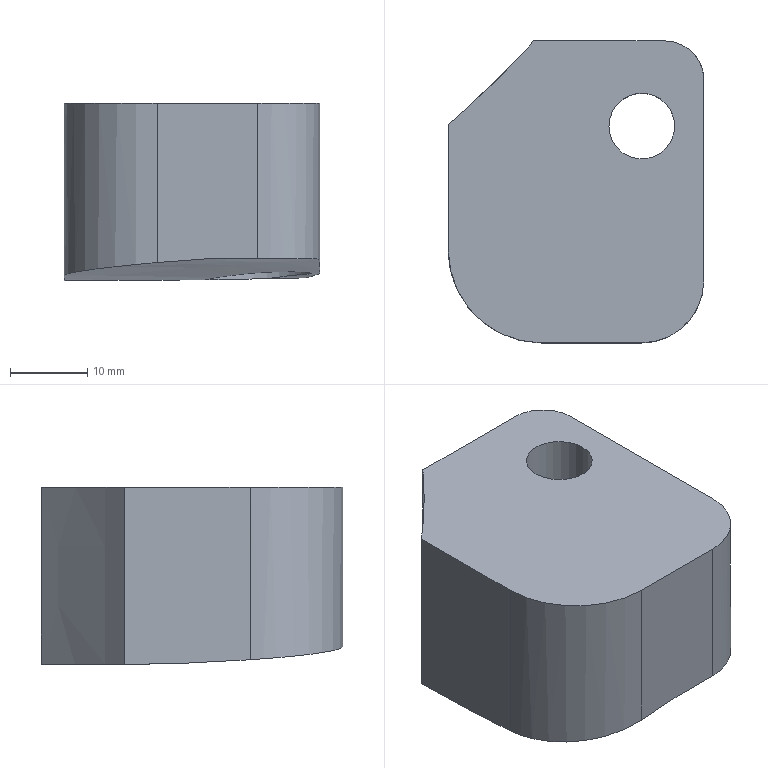Part | STEP file | gslz 2016.10.28-10_id774_x_t | 1 solid | 13 faces | box 33 x 39 x 22.871 mm | volume 23207 mm3 | plane 6 | cylinder 5 | spline 1 | other 1 | commonest cylinder face diameters 8.5 x1 10 x1 14 x1 16 x1 24 x1